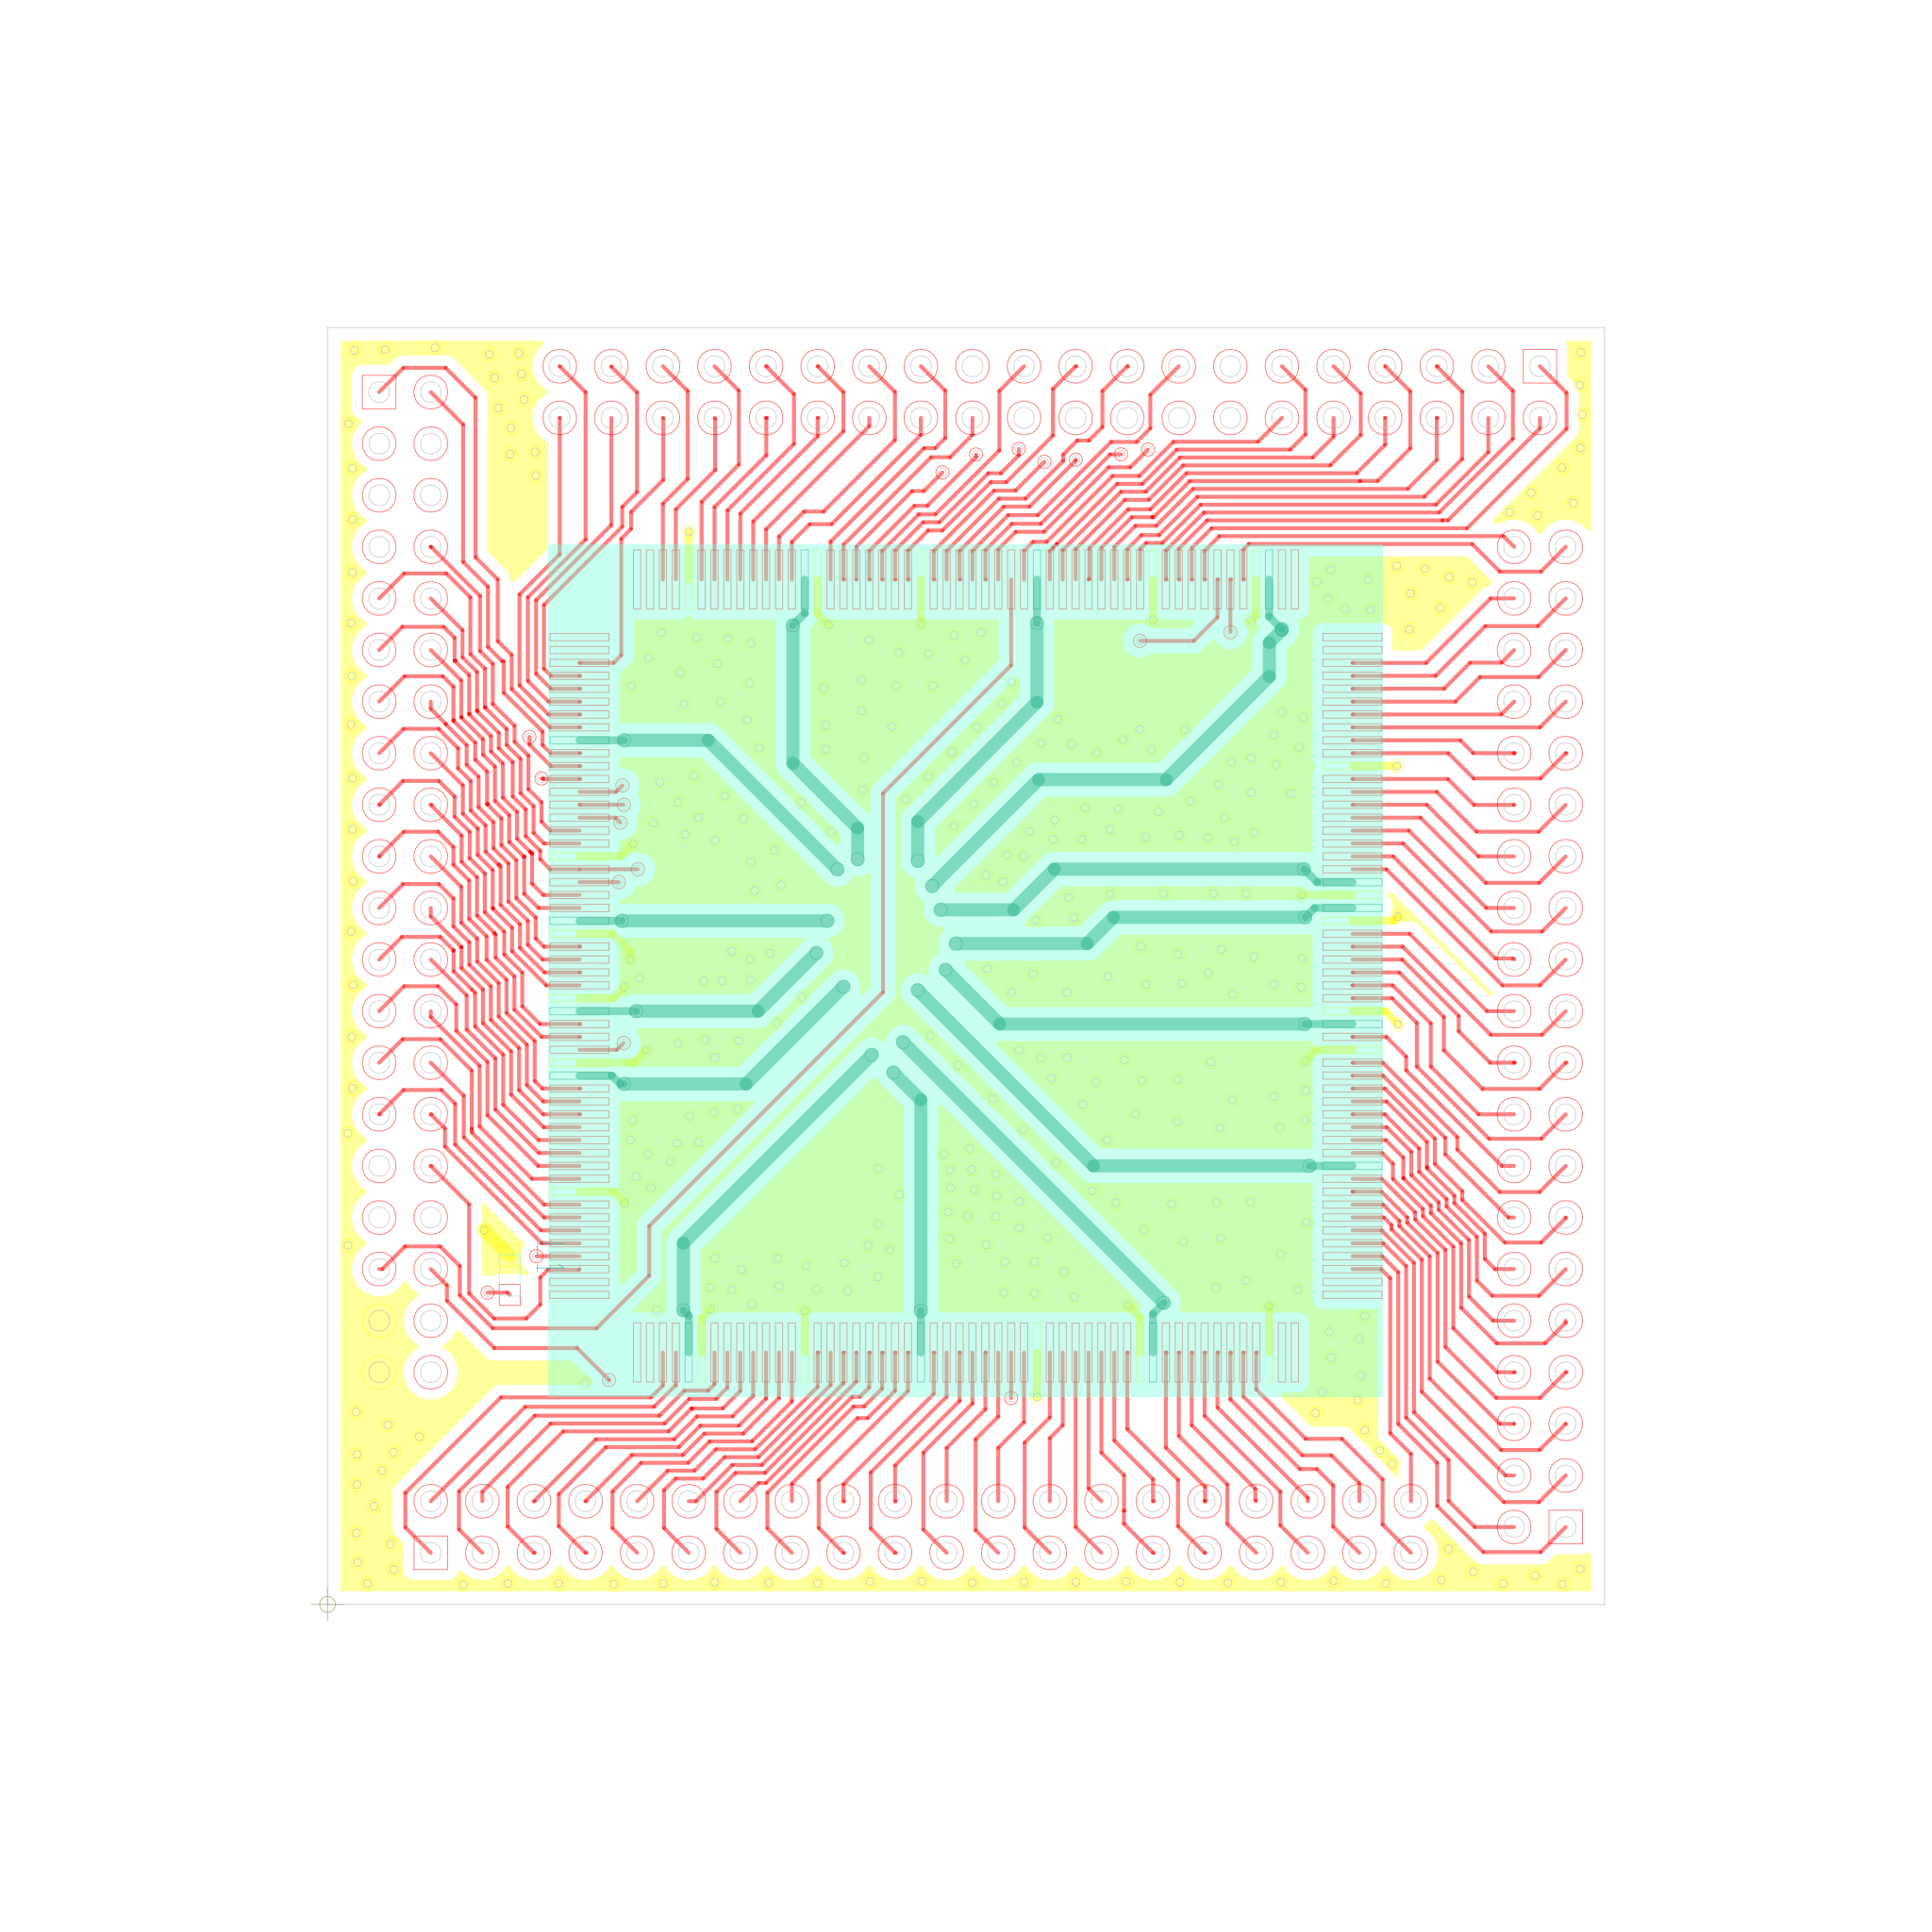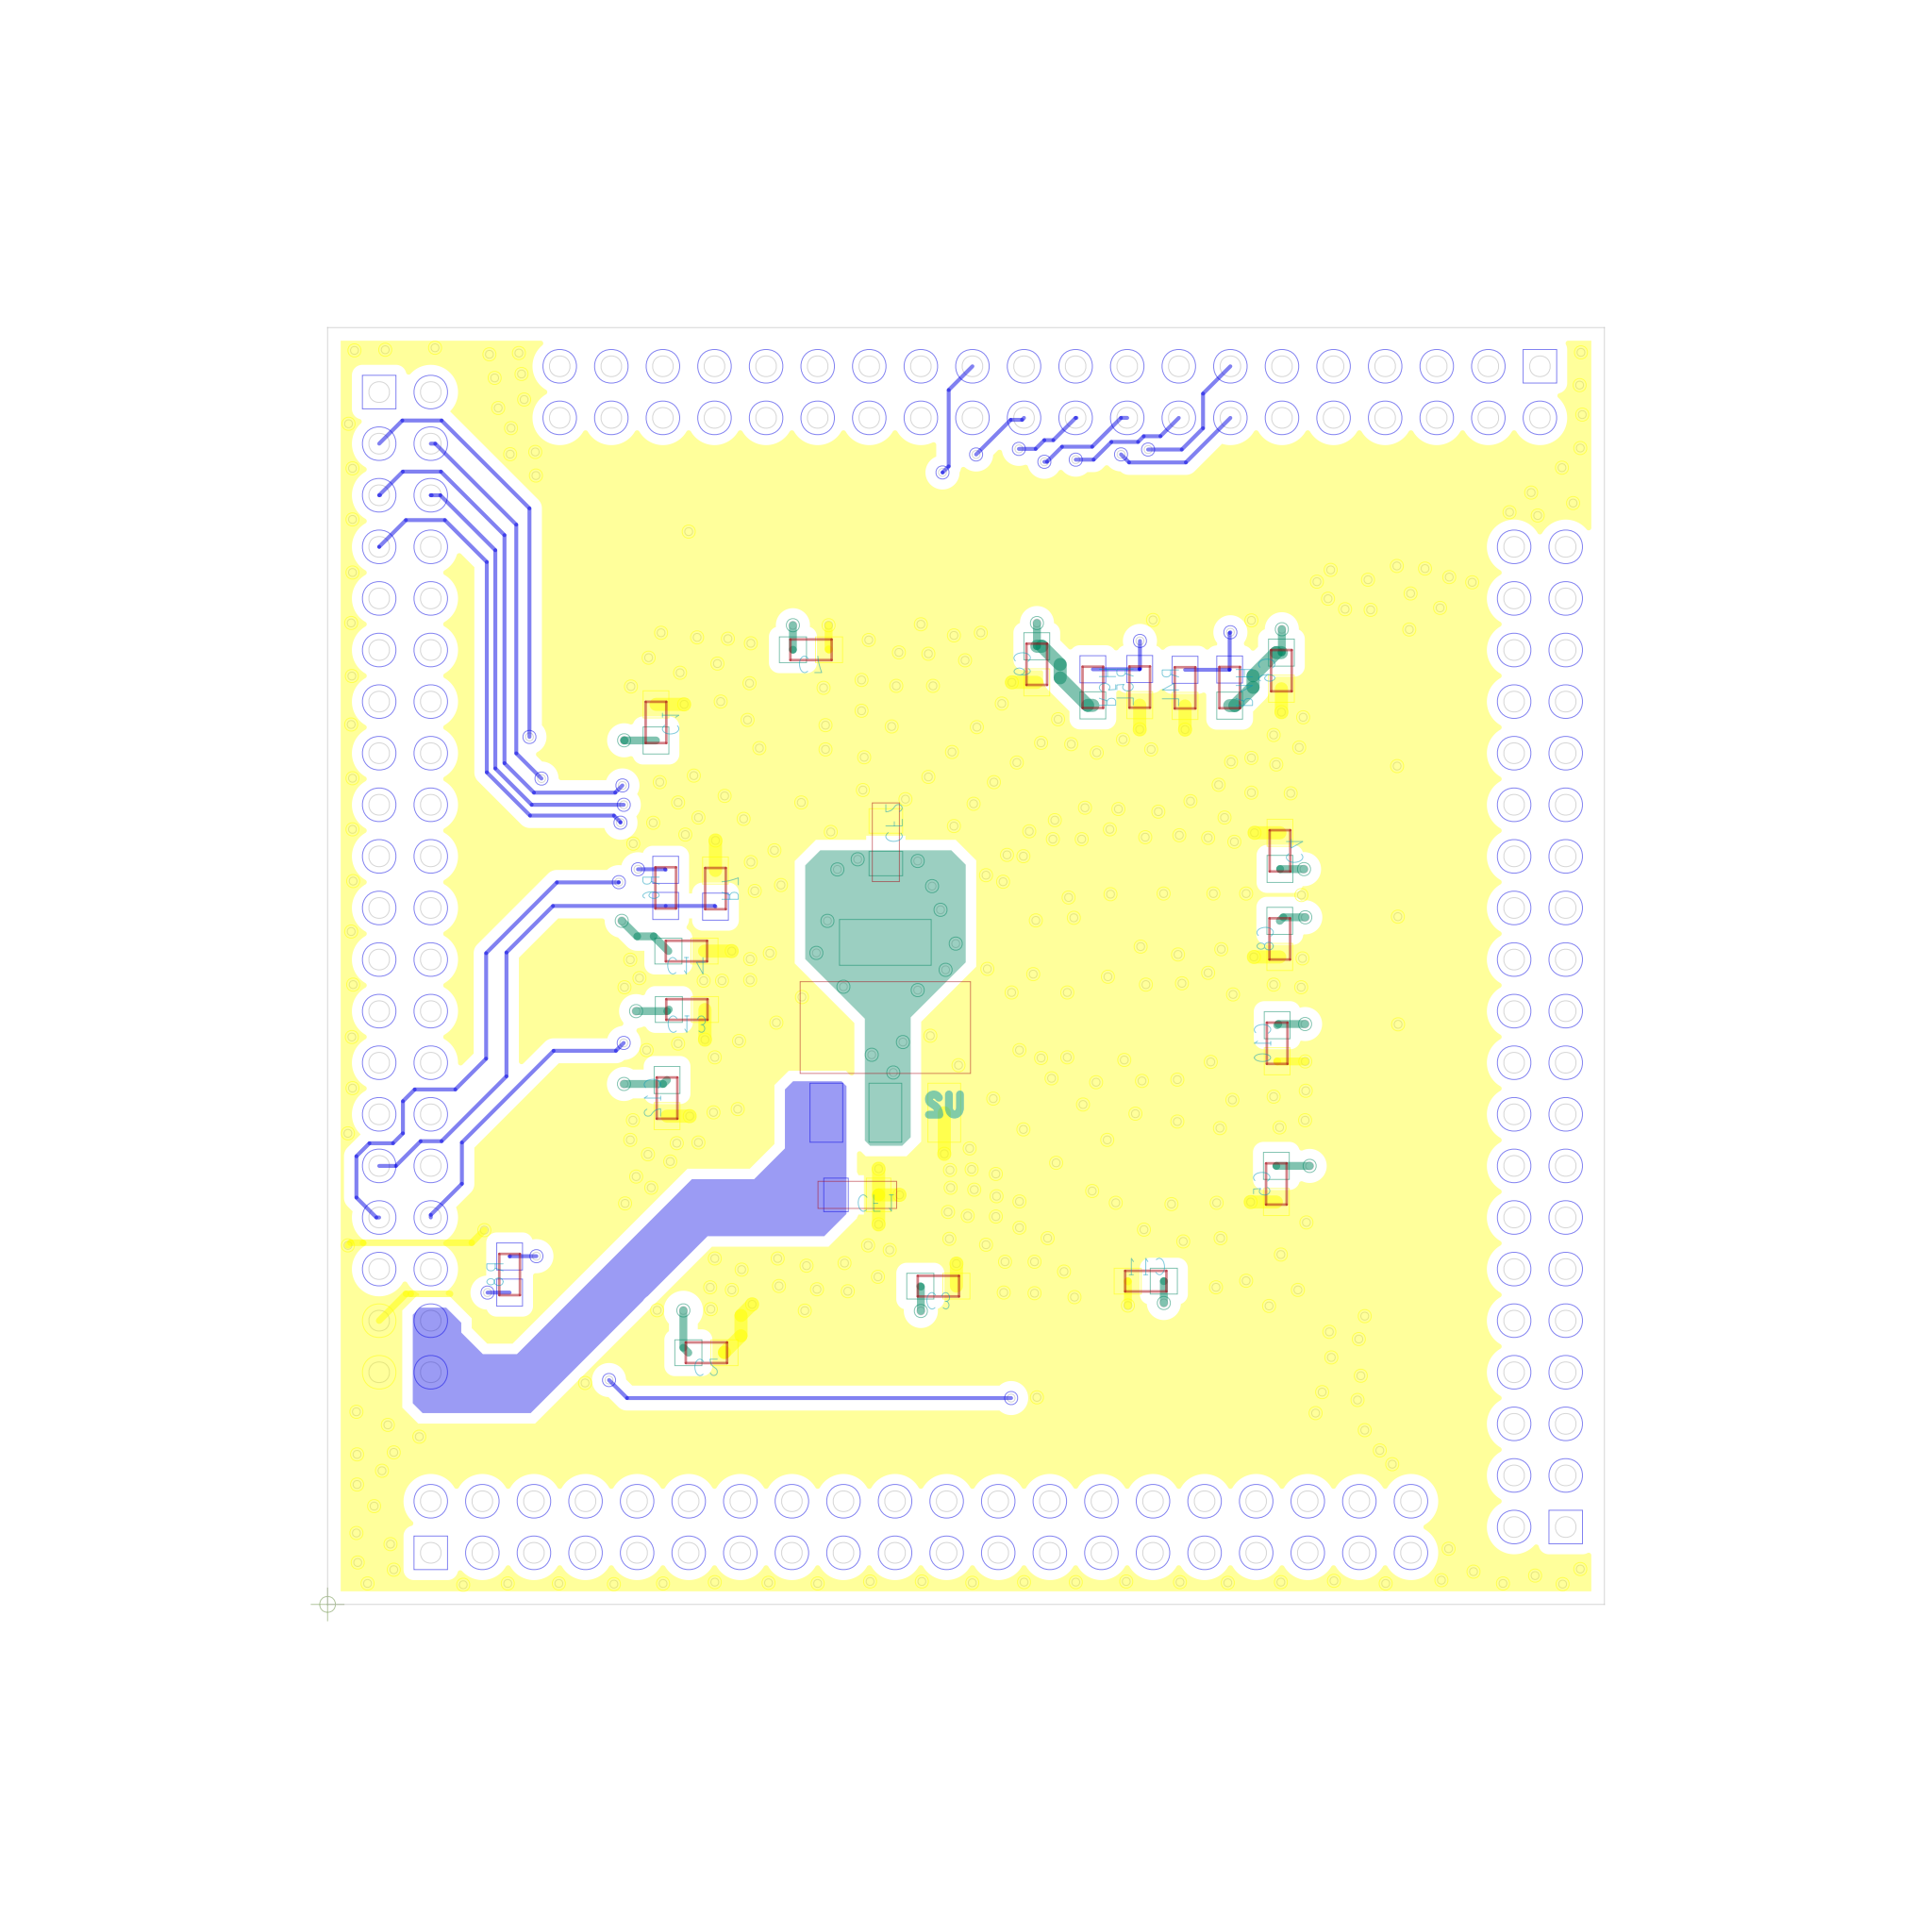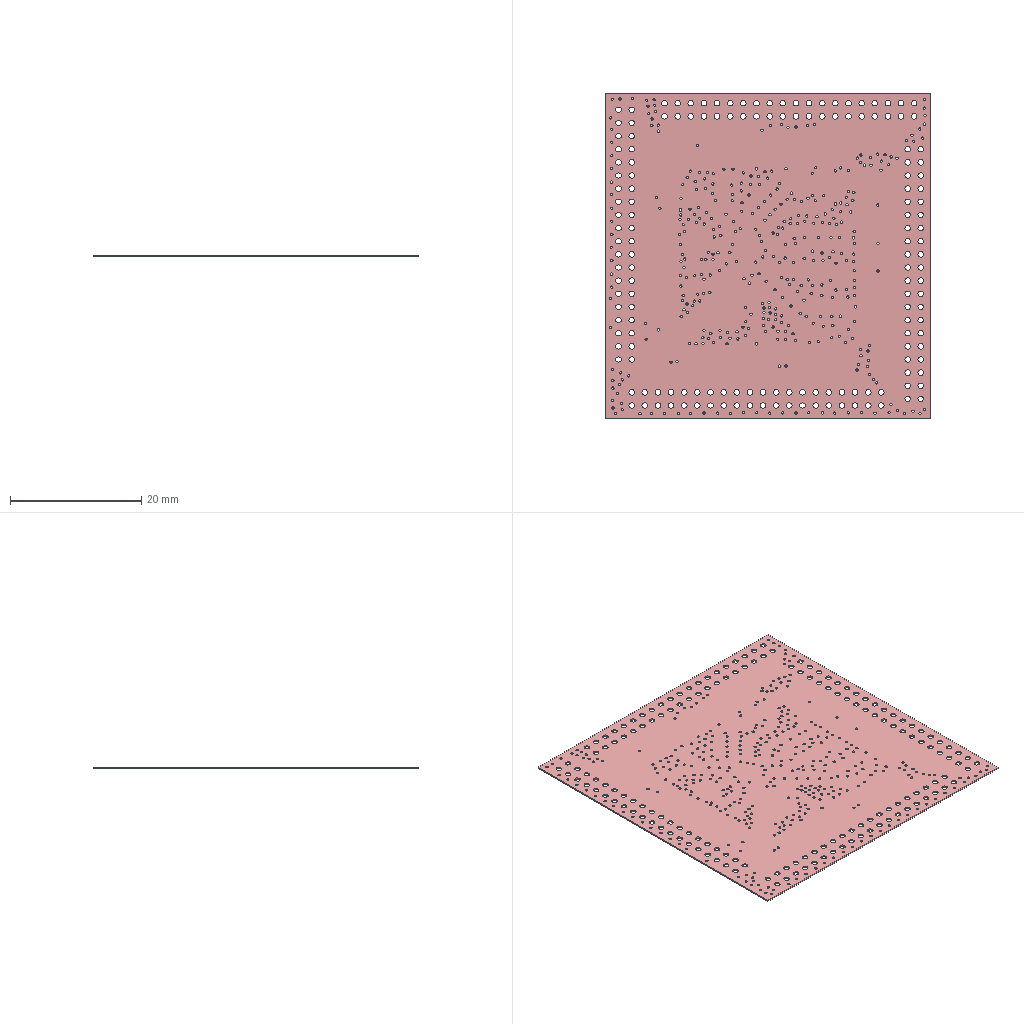Circuit board layout | Cadence Allegro | box 49.5 x 49.5 x 0.2 mm
Layer stack:
# Cadence Allegro layer stack of 2 (unit mm; from the constraint file cross-section; dielectric type: 0 not recorded (Allegro does not mark core vs prepreg), 3 surface material)
index,name,kind,layer,copper_thickness_mm,dielectric_type,dielectric_thickness_mm,dielectric_material,dielectric_constant
0,Top Surface,other,,,,,,
1,TOP,copper,TOP,0.0305,,,,
2,Dielectric1,dielectric,,,0,0.2032,FR-4,4.5
3,BOTTOM,copper,BOTTOM,0.0305,,,,
4,Bottom Surface,other,,,,,,
# drill layer pairs: low layer,high layer
drill_pair,TOP,BOTTOM
Part placement:
REFDES,COMP_VALUE,SYM_NAME,SYM_X,SYM_Y,SYM_ROTATE,SYM_MIRROR
C1,104 SMD0603,C0603,501.232,1346.193,270.000,YES
C2,104 SMD0603,C0603,578.224,384.138,180.000,YES
C3,104 SMD0603,C0603,932.244,485.748,180.000,YES
C4,104 SMD0603,C0603,1453.638,1150.177,270.000,YES
C5,104 SMD0603,C0603,1448.130,641.744,90.000,YES
C6,104 SMD0603,C0603,1455.846,1425.177,90.000,YES
C7,104 SMD0603,C0603,737.846,1457.094,180.000,YES
C8,104 SMD0603,C0603,1453.335,1015.772,90.000,YES
C9,104 SMD0603,C0603,1082.469,1434.894,90.000,YES
C10,104 SMD0603,C0603,1449.339,856.500,90.000,YES
C11,104 SMD0603,C0603,1248.795,493.394,0.000,YES
C12,104 SMD0603,C0603,518.126,772.807,90.000,YES
C13,104 SMD0603,C0603,548.421,908.012,180.000,YES
C14,104 SMD0603,C0603,547.736,997.169,180.000,YES
CF1,106 SMD0805,C0805,808.547,625.063,180.000,YES
CF2,106 SMD0805,C0805,852.087,1163.280,270.000,YES
J1,HEADER_20X2_200_DIP,DIP_20X2_2MM,157.480,78.740,0.000,NO
J2,HEADER_20X2_200_DIP,DIP_20X2_2MM,1889.764,118.110,90.000,NO
J3,HEADER_20X2_200_DIP,DIP_20X2_2MM,1850.394,1889.764,180.000,NO
J4,HEADER_20X2_200_DIP,DIP_20X2_2MM,78.740,1850.394,270.000,NO
L1,LED SMD0603,LED_0603,278.094,502.413,270.000,NO
R4H,10K SMD0603,R0603,1376.846,1399.358,270.000,YES
R4L,10K SMD0603,R0603,1308.760,1398.937,90.000,YES
R5H,10K SMD0603,R0603,1168.043,1399.752,270.000,YES
R5L,10K SMD0603,R0603,1239.535,1400.150,90.000,YES
R6,10K SMD 0603,R0603,516.039,1093.634,90.000,YES
R7,10K SMD 0603,R0603,592.043,1092.563,270.000,YES
R8,1K SMD0603,R0603,277.831,503.484,90.000,YES
U1,PQFP-208_30X30,PQFP-208_30X30,974.409,974.409,90.000,NO
U2,LD1117 SOT-223,SOT-223,941.295,750.457,0.000,YES
Pad and via stacks, first 115 of 286 lines:
# Allegro (Cadence) via spans and padstacks; design units: ("mils" 3 1000)
# via spans: padstack,start_layer,end_layer,net_example,count
VIA12X20,ETCH/TOP,ETCH/BOTTOM,GND,388
# Allegro padstack definitions: name,start_layer,end_layer,drill,plating,holeType,type
PAD19,"ETCH/TOP","ETCH/TOP",0.0,"NON_PLATED","none","smd"
PAD13,"ETCH/TOP","ETCH/TOP",0.0,"NON_PLATED","none","smd"
PAD12,"ETCH/TOP","ETCH/TOP",0.0,"NON_PLATED","none","smd"
PAD17,"ETCH/TOP","ETCH/TOP",0.0,"NON_PLATED","none","smd"
PAD15,"ETCH/TOP","ETCH/TOP",0.0,"NON_PLATED","none","smd"
PAD16,"ETCH/TOP","ETCH/TOP",0.0,"NON_PLATED","none","smd"
PAD1,"ETCH/TOP","ETCH/TOP",0.0,"NON_PLATED","none","smd"
PAD46,"ETCH/TOP","ETCH/TOP",0.0,"NON_PLATED","none","smd"
PAD44,"ETCH/TOP","ETCH/TOP",0.0,"NON_PLATED","none","smd"
PAD8,"ETCH/TOP","ETCH/TOP",0.0,"NON_PLATED","none","smd"
PAD5,"ETCH/TOP","ETCH/TOP",0.0,"NON_PLATED","none","smd"
PAD9,"ETCH/TOP","ETCH/TOP",0.0,"NON_PLATED","none","smd"
PAD10,"ETCH/TOP","ETCH/TOP",0.0,"NON_PLATED","none","smd"
PAD25,"ETCH/TOP","ETCH/TOP",0.0,"NON_PLATED","none","smd"
PAD4,"ETCH/TOP","ETCH/TOP",0.0,"NON_PLATED","none","smd"
PAD7,"ETCH/TOP","ETCH/TOP",0.0,"NON_PLATED","none","smd"
PAD6,"ETCH/TOP","ETCH/TOP",0.0,"NON_PLATED","none","smd"
PAD3,"ETCH/TOP","ETCH/TOP",0.0,"NON_PLATED","none","smd"
PAD31,"ETCH/TOP","ETCH/TOP",0.0,"NON_PLATED","none","smd"
PAD22,"ETCH/TOP","ETCH/TOP",0.0,"NON_PLATED","none","smd"
PAD41,"ETCH/TOP","ETCH/TOP",0.0,"NON_PLATED","none","smd"
PAD42,"ETCH/TOP","ETCH/TOP",0.0,"NON_PLATED","none","smd"
PAD43,"ETCH/TOP","ETCH/TOP",0.0,"NON_PLATED","none","smd"
PAD45,"ETCH/TOP","ETCH/TOP",0.0,"NON_PLATED","none","smd"
PAD2,"ETCH/TOP","ETCH/TOP",0.0,"NON_PLATED","none","smd"
PAD14,"ETCH/TOP","ETCH/TOP",0.0,"NON_PLATED","none","smd"
PAD21,"ETCH/TOP","ETCH/TOP",0.0,"NON_PLATED","none","smd"
PAD28,"ETCH/TOP","ETCH/TOP",0.0,"NON_PLATED","none","smd"
PAD26,"ETCH/TOP","ETCH/TOP",0.0,"NON_PLATED","none","smd"
PAD27,"ETCH/TOP","ETCH/TOP",0.0,"NON_PLATED","none","smd"
PAD18,"ETCH/TOP","ETCH/TOP",0.0,"NON_PLATED","none","smd"
PAD29,"ETCH/TOP","ETCH/TOP",0.0,"NON_PLATED","none","smd"
PAD20,"ETCH/TOP","ETCH/TOP",0.0,"NON_PLATED","none","smd"
PAD39,"ETCH/TOP","ETCH/TOP",0.0,"NON_PLATED","none","smd"
PAD40,"ETCH/TOP","ETCH/TOP",0.0,"NON_PLATED","none","smd"
PAD30,"ETCH/TOP","ETCH/TOP",0.0,"NON_PLATED","none","smd"
PAD48,"ETCH/TOP","ETCH/TOP",0.0,"NON_PLATED","none","smd"
PAD47,"ETCH/TOP","ETCH/TOP",0.0,"NON_PLATED","none","smd"
PAD49,"ETCH/TOP","ETCH/TOP",0.0,"NON_PLATED","none","smd"
PAD50,"ETCH/TOP","ETCH/TOP",0.0,"NON_PLATED","none","smd"
PAD53,"ETCH/TOP","ETCH/TOP",0.0,"NON_PLATED","none","smd"
F45,"ETCH/TOP","ETCH/TOP",0.0,"NON_PLATED","none","smd"
R88X76,"ETCH/TOP","ETCH/TOP",0.0,"PLATED","none","smd"
R127X121,"ETCH/TOP","ETCH/TOP",0.0,"PLATED","none","smd"
R127X152,"ETCH/TOP","ETCH/TOP",0.0,"NON_PLATED","none","smd"
R14X25,"ETCH/TOP","ETCH/TOP",0.0,"NON_PLATED","none","smd"
R165X317,"ETCH/TOP","ETCH/TOP",0.0,"NON_PLATED","none","smd"
R259X218,"ETCH/TOP","ETCH/TOP",0.0,"NON_PLATED","none","smd"
R70X22,"ETCH/TOP","ETCH/TOP",0.0,"NON_PLATED","none","smd"
R75X85,"ETCH/TOP","ETCH/TOP",0.0,"NON_PLATED","none","smd"
Y5,"ETCH/TOP","ETCH/TOP",0.0,"NON_PLATED","none","smd"
R16X30,"ETCH/TOP","ETCH/TOP",0.0,"NON_PLATED","none","smd"
F62X58,"ETCH/TOP","ETCH/TOP",0.0,"PLATED","none","smd"
R15X28,"ETCH/TOP","ETCH/TOP",0.0,"NON_PLATED","none","smd"
R195X280,"ETCH/TOP","ETCH/TOP",0.0,"NON_PLATED","none","smd"
R45X200,"ETCH/TOP","ETCH/TOP",0.0,"NON_PLATED","none","smd"
R50X30,"ETCH/TOP","ETCH/TOP",0.0,"NON_PLATED","none","smd"
R31X24,"ETCH/TOP","ETCH/TOP",0.0,"NON_PLATED","none","smd"
R215X60,"ETCH/TOP","ETCH/TOP",0.0,"NON_PLATED","none","smd"
S17,"ETCH/TOP","ETCH/TOP",0.0,"NON_PLATED","none","smd"
R23X25,"ETCH/TOP","ETCH/TOP",0.0,"NON_PLATED","none","smd"
R19X32,"ETCH/TOP","ETCH/TOP",0.0,"NON_PLATED","none","smd"
R61X15,"ETCH/TOP","ETCH/TOP",0.0,"NON_PLATED","none","smd"
R45X150,"ETCH/TOP","ETCH/TOP",0.0,"NON_PLATED","none","smd"
R12X8,"ETCH/TOP","ETCH/TOP",0.0,"NON_PLATED","none","smd"
R91X127,"ETCH/TOP","ETCH/TOP",0.0,"NON_PLATED","none","smd"
S91,"ETCH/TOP","ETCH/TOP",0.0,"NON_PLATED","none","smd"
R55X99,"ETCH/TOP","ETCH/TOP",0.0,"NON_PLATED","none","smd"
R299X199,"ETCH/TOP","ETCH/TOP",0.0,"NON_PLATED","none","smd"
R114X165,"ETCH/TOP","ETCH/TOP",0.0,"NON_PLATED","none","smd"
R60X90,"ETCH/TOP","ETCH/TOP",0.0,"NON_PLATED","none","smd"
R6X10,"ETCH/TOP","ETCH/TOP",0.0,"NON_PLATED","none","smd"
Y10,"ETCH/TOP","ETCH/TOP",0.0,"NON_PLATED","none","smd"
R114X74,"ETCH/TOP","ETCH/TOP",0.0,"NON_PLATED","none","smd"
R30X130,"ETCH/TOP","ETCH/TOP",0.0,"PLATED","none","smd"
R50X127,"ETCH/TOP","ETCH/TOP",0.0,"NON_PLATED","none","smd"
R18X20,"ETCH/TOP","ETCH/TOP",0.0,"NON_PLATED","none","smd"
R60X71,"ETCH/TOP","ETCH/TOP",0.0,"NON_PLATED","none","smd"
R48X71,"ETCH/TOP","ETCH/TOP",0.0,"NON_PLATED","none","smd"
R80X30,"ETCH/TOP","ETCH/TOP",0.0,"PLATED","none","smd"
FLASH_0,"ETCH/TOP","ETCH/TOP",0.0,"PLATED","none","smd"
Y3,"ETCH/TOP","ETCH/TOP",0.0,"PLATED","none","smd"
R170X25,"ETCH/TOP","ETCH/TOP",0.0,"PLATED","none","smd"
R70X25,"ETCH/TOP","ETCH/TOP",0.0,"PLATED","none","smd"
R43X14,"ETCH/TOP","ETCH/TOP",0.0,"PLATED","none","smd"
R33X10,"ETCH/TOP","ETCH/TOP",0.0,"PLATED","none","smd"
R636X23,"ETCH/TOP","ETCH/TOP",0.0,"PLATED","none","smd"
R155X35,"ETCH/TOP","ETCH/TOP",0.0,"PLATED","none","smd"
R60X20,"ETCH/TOP","ETCH/TOP",0.0,"PLATED","none","smd"
R120X70,"ETCH/TOP","ETCH/TOP",0.0,"PLATED","none","smd"
SMD0_45R,"ETCH/TOP","ETCH/TOP",0.0,"PLATED","none","smd"
Y42,"ETCH/TOP","ETCH/TOP",0.0,"PLATED","none","smd"
R85X65,"ETCH/TOP","ETCH/TOP",0.0,"PLATED","none","smd"
Y30,"ETCH/TOP","ETCH/TOP",0.0,"PLATED","none","smd"
R53X20,"ETCH/TOP","ETCH/TOP",0.0,"PLATED","none","smd"
R55X40,"ETCH/TOP","ETCH/TOP",0.0,"PLATED","none","smd"
R155X25,"ETCH/TOP","ETCH/TOP",0.0,"PLATED","none","smd"
F17X17,"ETCH/TOP","ETCH/TOP",0.0,"PLATED","none","smd"
F89X32,"ETCH/TOP","ETCH/TOP",0.0,"PLATED","none","smd"
R8X2,"ETCH/TOP","ETCH/TOP",0.0,"PLATED","none","smd"
SMD40X20,"ETCH/TOP","ETCH/TOP",0.0,"PLATED","none","smd"
R340X185,"ETCH/TOP","ETCH/TOP",0.0,"PLATED","none","smd"
R27X10,"ETCH/TOP","ETCH/TOP",0.0,"PLATED","none","smd"
R22X11,"ETCH/TOP","ETCH/TOP",0.0,"PLATED","none","smd"
R32X36,"ETCH/TOP","ETCH/TOP",0.0,"PLATED","none","smd"
S21X20,"ETCH/TOP","ETCH/TOP",0.0,"PLATED","none","smd"
R13X10,"ETCH/TOP","ETCH/TOP",0.0,"PLATED","none","smd"
R75X28,"ETCH/TOP","ETCH/TOP",0.0,"PLATED","none","smd"
R25X15,"ETCH/TOP","ETCH/TOP",0.0,"NON_PLATED","none","smd"
C0_5,"ETCH/TOP","ETCH/TOP",0.0,"PLATED","none","smd"
S437,"ETCH/TOP","ETCH/TOP",0.0,"PLATED","none","smd"
Design rules, without the lines most boards share, first 14 of 31 lines:
# Cadence Allegro design rules of 2 (from the Constraint Manager export 2-constraints.dcfx, design unit mil; typed fields in mm)
# columns: name | kind | enabled | priority | scope1 | scope2 | descriptor | typed fields (field=value)
# Allegro precedence (priority 1 wins): 1 Region class-to-class, 2 Region class, 3 Region, 4 class-to-class, 5 DiffPair/Bus/NetGroup override, 6 NetClass, 7 constraint set (CSet) default
# per-layer values are written LAYER=value in the descriptor and LAYER:mm in the typed field; a maximum of 0 means no limit set
# --- net classes (and buses / net groups) ---
PHY_R | NetClass | enabled | 6 | no members | All | Net Class (members: 0) |
PHY_T | NetClass | enabled | 6 | no members | All | Net Class (members: 0) |
DDR3_A | NetClass | enabled | 6 | no members | All | Net Class (members: 0) |
DDR3_DQH1 | NetClass | enabled | 6 | no members | All | Net Class (members: 0) |
DDR3_DQL1 | NetClass | enabled | 6 | no members | All | Net Class (members: 0) |
DDR3_DQH0 | NetClass | enabled | 6 | no members | All | Net Class (members: 0) |
DDR3_DQL0 | NetClass | enabled | 6 | no members | All | Net Class (members: 0) |
# --- track widths, neck and differential-pair gap (physical constraint sets) ---
DEFAULT | PhysicalCSet | enabled | 7 | Design default | All | Physical Constraint (Min Line Width=6mil) (Max Line Width=0mil) (Min Neck Width=6mil) (Max Neck Length=0mil) (DiffPair Primary Gap=6mil) (DiffPair Neck Gap=0mil) (DiffPair Min Space=0mil) (DiffPair Coupled +Tol=0mil) (DiffPair Coupled -Tol=0mil) (Min BB Via Stagger=5mil) (Max BB Via Stagger=0mil) (T-junctions=ANYWHERE) (Pad-pad direct connect=ALL_ALLOWED) (Allowed vias=VIA12X20) | min_line_width=0.1524 min_neck_width=0.1524 min_bvia_stagger=0.127 max_bvia_stagger=0 ts_allowed=ANYWHERE diffp_primary_gap=0.1524 diffp_neck_gap=0 max_line_width=0 maximum_neck_length=0 pad_pad_direct_connect=ALL_ALLOWED allow_on_etch_subclass=TRUE diffp_coupled_plus=0 diffp_coupled_minus=0 diffp_min_space=0 vias=VIA12X20